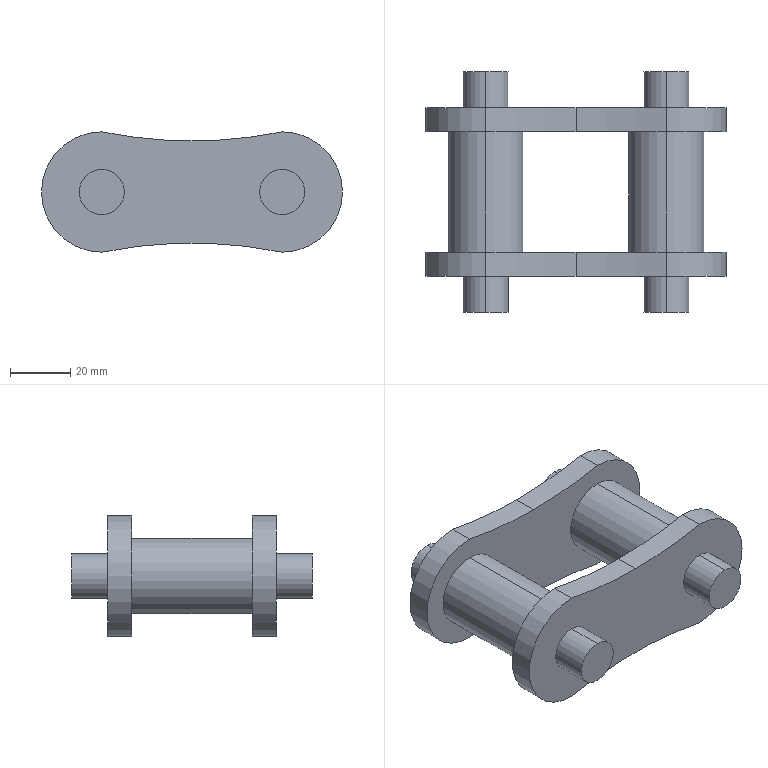Part | SolidWorks | features ICE 2, LPattern 2, RefPoint 2, Extrusion 1 | 1 solid | 30 faces | box 100 x 80 x 40 mm | volume 102371 mm3 | cylinder 22 | plane 8 | commonest cylinder face diameters 15 x8 300 x6 25 x4 40 x4
STEP:
#1=CARTESIAN_POINT('',(0.,0.,-7.5));
#2=VERTEX_POINT('',#1);
#3=CARTESIAN_POINT('',(0.,0.,7.5));
#4=VERTEX_POINT('',#3);
#5=CARTESIAN_POINT('',(0.,0.,0.));
#6=DIRECTION('',(0.,-1.,0.));
#7=DIRECTION('',(0.,0.,1.));
#8=AXIS2_PLACEMENT_3D('',#5,#6,#7);
#9=CIRCLE('',#8,7.5);
#10=EDGE_CURVE('',#2,#4,#9,.T.);
#11=ORIENTED_EDGE('',*,*,#10,.T.);
#12=CARTESIAN_POINT('',(0.,-12.,7.5));
#13=VERTEX_POINT('',#12);
#14=CARTESIAN_POINT('',(0.,0.,7.5));
#15=DIRECTION('',(0.,-1.,0.));
#16=VECTOR('',#15,1000.);
#17=LINE('',#14,#16);
#18=EDGE_CURVE('',#4,#13,#17,.T.);
#19=ORIENTED_EDGE('',*,*,#18,.T.);
#20=CARTESIAN_POINT('',(0.,-12.,-7.5));
#21=VERTEX_POINT('',#20);
#22=CARTESIAN_POINT('',(0.,-12.,0.));
#23=DIRECTION('',(0.,1.,0.));
#24=DIRECTION('',(0.,0.,1.));
#25=AXIS2_PLACEMENT_3D('',#22,#23,#24);
#26=CIRCLE('',#25,7.5);
#27=EDGE_CURVE('',#13,#21,#26,.T.);
#28=ORIENTED_EDGE('',*,*,#27,.T.);
#29=CARTESIAN_POINT('',(0.,0.,-7.5));
#30=DIRECTION('',(0.,-1.,0.));
#31=VECTOR('',#30,1000.);
#32=LINE('',#29,#31);
#33=EDGE_CURVE('',#2,#21,#32,.T.);
#34=ORIENTED_EDGE('',*,*,#33,.F.);
#35=EDGE_LOOP('',(#11,#19,#28,#34));
#36=FACE_OUTER_BOUND('',#35,.T.);
#37=CARTESIAN_POINT('',(0.,0.,0.));
#38=DIRECTION('',(0.,-1.,0.));
#39=DIRECTION('',(0.,0.,-1.));
#40=AXIS2_PLACEMENT_3D('',#37,#38,#39);
#41=CYLINDRICAL_SURFACE('',#40,7.5);
#42=ADVANCED_FACE('',(#36),#41,.T.);
#43=CARTESIAN_POINT('',(60.,0.,-7.5));
#44=VERTEX_POINT('',#43);
#45=CARTESIAN_POINT('',(60.,0.,7.5));
#46=VERTEX_POINT('',#45);
#47=CARTESIAN_POINT('',(60.,0.,0.));
#48=DIRECTION('',(0.,-1.,0.));
#49=DIRECTION('',(0.,0.,1.));
#50=AXIS2_PLACEMENT_3D('',#47,#48,#49);
#51=CIRCLE('',#50,7.5);
#52=EDGE_CURVE('',#44,#46,#51,.T.);
#53=ORIENTED_EDGE('',*,*,#52,.T.);
#54=CARTESIAN_POINT('',(60.,-12.,7.5));
#55=VERTEX_POINT('',#54);
#56=CARTESIAN_POINT('',(60.,0.,7.5));
#57=DIRECTION('',(0.,-1.,0.));
#58=VECTOR('',#57,1000.);
#59=LINE('',#56,#58);
#60=EDGE_CURVE('',#46,#55,#59,.T.);
#61=ORIENTED_EDGE('',*,*,#60,.T.);
#62=CARTESIAN_POINT('',(60.,-12.,-7.5));
#63=VERTEX_POINT('',#62);
#64=CARTESIAN_POINT('',(60.,-12.,0.));
#65=DIRECTION('',(0.,1.,0.));
#66=DIRECTION('',(0.,0.,1.));
#67=AXIS2_PLACEMENT_3D('',#64,#65,#66);
#68=CIRCLE('',#67,7.5);
#69=EDGE_CURVE('',#55,#63,#68,.T.);
#70=ORIENTED_EDGE('',*,*,#69,.T.);
#71=CARTESIAN_POINT('',(60.,0.,-7.5));
#72=DIRECTION('',(0.,-1.,0.));
#73=VECTOR('',#72,1000.);
#74=LINE('',#71,#73);
#75=EDGE_CURVE('',#44,#63,#74,.T.);
#76=ORIENTED_EDGE('',*,*,#75,.F.);
#77=EDGE_LOOP('',(#53,#61,#70,#76));
#78=FACE_OUTER_BOUND('',#77,.T.);
#79=CARTESIAN_POINT('',(60.,0.,0.));
#80=DIRECTION('',(0.,-1.,0.));
#81=DIRECTION('',(0.,0.,-1.));
#82=AXIS2_PLACEMENT_3D('',#79,#80,#81);
#83=CYLINDRICAL_SURFACE('',#82,7.5);
#84=ADVANCED_FACE('',(#78),#83,.T.);
#85=CARTESIAN_POINT('',(0.,68.,7.5));
#86=VERTEX_POINT('',#85);
#87=CARTESIAN_POINT('',(0.,68.,-7.5));
#88=VERTEX_POINT('',#87);
#89=CARTESIAN_POINT('',(0.,68.,0.));
#90=DIRECTION('',(0.,1.,0.));
#91=DIRECTION('',(0.,0.,1.));
#92=AXIS2_PLACEMENT_3D('',#89,#90,#91);
#93=CIRCLE('',#92,7.5);
#94=EDGE_CURVE('',#86,#88,#93,.T.);
#95=ORIENTED_EDGE('',*,*,#94,.F.);
#96=CARTESIAN_POINT('',(0.,56.,7.5));
#97=VERTEX_POINT('',#96);
#98=CARTESIAN_POINT('',(0.,68.,7.5));
#99=DIRECTION('',(0.,-1.,0.));
#100=VECTOR('',#99,1000.);
#101=LINE('',#98,#100);
#102=EDGE_CURVE('',#86,#97,#101,.T.);
#103=ORIENTED_EDGE('',*,*,#102,.T.);
#104=CARTESIAN_POINT('',(0.,56.,-7.5));
#105=VERTEX_POINT('',#104);
#106=CARTESIAN_POINT('',(0.,56.,0.));
#107=DIRECTION('',(0.,1.,0.));
#108=DIRECTION('',(0.,0.,1.));
#109=AXIS2_PLACEMENT_3D('',#106,#107,#108);
#110=CIRCLE('',#109,7.5);
#111=EDGE_CURVE('',#97,#105,#110,.T.);
#112=ORIENTED_EDGE('',*,*,#111,.T.);
#113=CARTESIAN_POINT('',(0.,68.,-7.5));
#114=DIRECTION('',(0.,-1.,0.));
#115=VECTOR('',#114,1000.);
#116=LINE('',#113,#115);
#117=EDGE_CURVE('',#88,#105,#116,.T.);
#118=ORIENTED_EDGE('',*,*,#117,.F.);
#119=EDGE_LOOP('',(#95,#103,#112,#118));
#120=FACE_OUTER_BOUND('',#119,.T.);
#121=CARTESIAN_POINT('',(0.,68.,0.));
#122=DIRECTION('',(0.,-1.,0.));
#123=DIRECTION('',(0.,0.,-1.));
#124=AXIS2_PLACEMENT_3D('',#121,#122,#123);
#125=CYLINDRICAL_SURFACE('',#124,7.5);
#126=ADVANCED_FACE('',(#120),#125,.T.);
#127=CARTESIAN_POINT('',(60.,68.,7.5));
#128=VERTEX_POINT('',#127);
#129=CARTESIAN_POINT('',(60.,68.,-7.5));
#130=VERTEX_POINT('',#129);
#131=CARTESIAN_POINT('',(60.,68.,0.));
#132=DIRECTION('',(0.,1.,0.));
#133=DIRECTION('',(0.,0.,1.));
#134=AXIS2_PLACEMENT_3D('',#131,#132,#133);
#135=CIRCLE('',#134,7.5);
#136=EDGE_CURVE('',#128,#130,#135,.T.);
#137=ORIENTED_EDGE('',*,*,#136,.F.);
#138=CARTESIAN_POINT('',(60.,56.,7.5));
#139=VERTEX_POINT('',#138);
#140=CARTESIAN_POINT('',(60.,68.,7.5));
#141=DIRECTION('',(0.,-1.,0.));
#142=VECTOR('',#141,1000.);
#143=LINE('',#140,#142);
#144=EDGE_CURVE('',#128,#139,#143,.T.);
#145=ORIENTED_EDGE('',*,*,#144,.T.);
#146=CARTESIAN_POINT('',(60.,56.,-7.5));
#147=VERTEX_POINT('',#146);
#148=CARTESIAN_POINT('',(60.,56.,0.));
#149=DIRECTION('',(0.,1.,0.));
#150=DIRECTION('',(0.,0.,1.));
#151=AXIS2_PLACEMENT_3D('',#148,#149,#150);
#152=CIRCLE('',#151,7.5);
#153=EDGE_CURVE('',#139,#147,#152,.T.);
#154=ORIENTED_EDGE('',*,*,#153,.T.);
#155=CARTESIAN_POINT('',(60.,68.,-7.5));
#156=DIRECTION('',(0.,-1.,0.));
#157=VECTOR('',#156,1000.);
#158=LINE('',#155,#157);
#159=EDGE_CURVE('',#130,#147,#158,.T.);
#160=ORIENTED_EDGE('',*,*,#159,.F.);
#161=EDGE_LOOP('',(#137,#145,#154,#160));
#162=FACE_OUTER_BOUND('',#161,.T.);
#163=CARTESIAN_POINT('',(60.,68.,0.));
#164=DIRECTION('',(0.,-1.,0.));
#165=DIRECTION('',(0.,0.,-1.));
#166=AXIS2_PLACEMENT_3D('',#163,#164,#165);
#167=CYLINDRICAL_SURFACE('',#166,7.5);
#168=ADVANCED_FACE('',(#162),#167,.T.);
#169=CARTESIAN_POINT('',(30.,56.,16.969));
#170=VERTEX_POINT('',#169);
#171=CARTESIAN_POINT('',(60.,56.,20.));
#172=VERTEX_POINT('',#171);
#173=CARTESIAN_POINT('',(30.,56.,166.969));
#174=DIRECTION('',(0.,-1.,0.));
#175=DIRECTION('',(0.,0.,-1.));
#176=AXIS2_PLACEMENT_3D('',#173,#174,#175);
#177=CIRCLE('',#176,150.);
#178=EDGE_CURVE('',#170,#172,#177,.T.);
#179=ORIENTED_EDGE('',*,*,#178,.F.);
#180=CARTESIAN_POINT('',(30.,48.,16.969));
#181=VERTEX_POINT('',#180);
#182=CARTESIAN_POINT('',(30.,56.,16.969));
#183=DIRECTION('',(0.,-1.,0.));
#184=VECTOR('',#183,1000.);
#185=LINE('',#182,#184);
#186=EDGE_CURVE('',#170,#181,#185,.T.);
#187=ORIENTED_EDGE('',*,*,#186,.T.);
#188=CARTESIAN_POINT('',(60.,48.,20.));
#189=VERTEX_POINT('',#188);
#190=CARTESIAN_POINT('',(30.,48.,166.969));
#191=DIRECTION('',(0.,-1.,0.));
#192=DIRECTION('',(0.,0.,-1.));
#193=AXIS2_PLACEMENT_3D('',#190,#191,#192);
#194=CIRCLE('',#193,150.);
#195=EDGE_CURVE('',#181,#189,#194,.T.);
#196=ORIENTED_EDGE('',*,*,#195,.T.);
#197=CARTESIAN_POINT('',(60.,56.,20.));
#198=DIRECTION('',(0.,-1.,0.));
#199=VECTOR('',#198,1000.);
#200=LINE('',#197,#199);
#201=EDGE_CURVE('',#172,#189,#200,.T.);
#202=ORIENTED_EDGE('',*,*,#201,.F.);
#203=EDGE_LOOP('',(#179,#187,#196,#202));
#204=FACE_OUTER_BOUND('',#203,.T.);
#205=CARTESIAN_POINT('',(30.,56.,166.969));
#206=DIRECTION('',(0.,-1.,0.));
#207=DIRECTION('',(0.,0.,-1.));
#208=AXIS2_PLACEMENT_3D('',#205,#206,#207);
#209=CYLINDRICAL_SURFACE('',#208,150.);
#210=ADVANCED_FACE('',(#204),#209,.F.);
#211=CARTESIAN_POINT('',(0.,48.,12.5));
#212=VERTEX_POINT('',#211);
#213=CARTESIAN_POINT('',(0.,48.,-12.5));
#214=VERTEX_POINT('',#213);
#215=CARTESIAN_POINT('',(0.,48.,0.));
#216=DIRECTION('',(0.,1.,0.));
#217=DIRECTION('',(0.,0.,1.));
#218=AXIS2_PLACEMENT_3D('',#215,#216,#217);
#219=CIRCLE('',#218,12.5);
#220=EDGE_CURVE('',#212,#214,#219,.T.);
#221=ORIENTED_EDGE('',*,*,#220,.F.);
#222=CARTESIAN_POINT('',(0.,8.,12.5));
#223=VERTEX_POINT('',#222);
#224=CARTESIAN_POINT('',(0.,48.,12.5));
#225=DIRECTION('',(0.,-1.,0.));
#226=VECTOR('',#225,1000.);
#227=LINE('',#224,#226);
#228=EDGE_CURVE('',#212,#223,#227,.T.);
#229=ORIENTED_EDGE('',*,*,#228,.T.);
#230=CARTESIAN_POINT('',(0.,8.,-12.5));
#231=VERTEX_POINT('',#230);
#232=CARTESIAN_POINT('',(0.,8.,0.));
#233=DIRECTION('',(0.,1.,0.));
#234=DIRECTION('',(0.,0.,1.));
#235=AXIS2_PLACEMENT_3D('',#232,#233,#234);
#236=CIRCLE('',#235,12.5);
#237=EDGE_CURVE('',#223,#231,#236,.T.);
#238=ORIENTED_EDGE('',*,*,#237,.T.);
#239=CARTESIAN_POINT('',(0.,48.,-12.5));
#240=DIRECTION('',(0.,-1.,0.));
#241=VECTOR('',#240,1000.);
#242=LINE('',#239,#241);
#243=EDGE_CURVE('',#214,#231,#242,.T.);
#244=ORIENTED_EDGE('',*,*,#243,.F.);
#245=EDGE_LOOP('',(#221,#229,#238,#244));
#246=FACE_OUTER_BOUND('',#245,.T.);
#247=CARTESIAN_POINT('',(0.,48.,0.));
#248=DIRECTION('',(0.,-1.,0.));
#249=DIRECTION('',(0.,0.,-1.));
#250=AXIS2_PLACEMENT_3D('',#247,#248,#249);
#251=CYLINDRICAL_SURFACE('',#250,12.5);
#252=ADVANCED_FACE('',(#246),#251,.T.);
#253=CARTESIAN_POINT('',(60.,48.,12.5));
#254=VERTEX_POINT('',#253);
#255=CARTESIAN_POINT('',(60.,48.,-12.5));
#256=VERTEX_POINT('',#255);
#257=CARTESIAN_POINT('',(60.,48.,0.));
#258=DIRECTION('',(0.,1.,0.));
#259=DIRECTION('',(0.,0.,1.));
#260=AXIS2_PLACEMENT_3D('',#257,#258,#259);
#261=CIRCLE('',#260,12.5);
#262=EDGE_CURVE('',#254,#256,#261,.T.);
#263=ORIENTED_EDGE('',*,*,#262,.F.);
#264=CARTESIAN_POINT('',(60.,8.,12.5));
#265=VERTEX_POINT('',#264);
#266=CARTESIAN_POINT('',(60.,48.,12.5));
#267=DIRECTION('',(0.,-1.,0.));
#268=VECTOR('',#267,1000.);
#269=LINE('',#266,#268);
#270=EDGE_CURVE('',#254,#265,#269,.T.);
#271=ORIENTED_EDGE('',*,*,#270,.T.);
#272=CARTESIAN_POINT('',(60.,8.,-12.5));
#273=VERTEX_POINT('',#272);
#274=CARTESIAN_POINT('',(60.,8.,0.));
#275=DIRECTION('',(0.,1.,0.));
#276=DIRECTION('',(0.,0.,1.));
#277=AXIS2_PLACEMENT_3D('',#274,#275,#276);
#278=CIRCLE('',#277,12.5);
#279=EDGE_CURVE('',#265,#273,#278,.T.);
#280=ORIENTED_EDGE('',*,*,#279,.T.);
#281=CARTESIAN_POINT('',(60.,48.,-12.5));
#282=DIRECTION('',(0.,-1.,0.));
#283=VECTOR('',#282,1000.);
#284=LINE('',#281,#283);
#285=EDGE_CURVE('',#256,#273,#284,.T.);
#286=ORIENTED_EDGE('',*,*,#285,.F.);
#287=EDGE_LOOP('',(#263,#271,#280,#286));
#288=FACE_OUTER_BOUND('',#287,.T.);
#289=CARTESIAN_POINT('',(60.,48.,0.));
#290=DIRECTION('',(0.,-1.,0.));
#291=DIRECTION('',(0.,0.,-1.));
#292=AXIS2_PLACEMENT_3D('',#289,#290,#291);
#293=CYLINDRICAL_SURFACE('',#292,12.5);
#294=ADVANCED_FACE('',(#288),#293,.T.);
#295=CARTESIAN_POINT('',(30.,8.,16.969));
#296=VERTEX_POINT('',#295);
#297=CARTESIAN_POINT('',(60.,8.,20.));
#298=VERTEX_POINT('',#297);
#299=CARTESIAN_POINT('',(30.,8.,166.969));
#300=DIRECTION('',(0.,-1.,0.));
#301=DIRECTION('',(0.,0.,-1.));
#302=AXIS2_PLACEMENT_3D('',#299,#300,#301);
#303=CIRCLE('',#302,150.);
#304=EDGE_CURVE('',#296,#298,#303,.T.);
#305=ORIENTED_EDGE('',*,*,#304,.F.);
#306=CARTESIAN_POINT('',(30.,0.,16.969));
#307=VERTEX_POINT('',#306);
#308=CARTESIAN_POINT('',(30.,8.,16.969));
#309=DIRECTION('',(0.,-1.,0.));
#310=VECTOR('',#309,1000.);
#311=LINE('',#308,#310);
#312=EDGE_CURVE('',#296,#307,#311,.T.);
#313=ORIENTED_EDGE('',*,*,#312,.T.);
#314=CARTESIAN_POINT('',(60.,0.,20.));
#315=VERTEX_POINT('',#314);
#316=CARTESIAN_POINT('',(30.,0.,166.969));
#317=DIRECTION('',(0.,-1.,0.));
#318=DIRECTION('',(0.,0.,-1.));
#319=AXIS2_PLACEMENT_3D('',#316,#317,#318);
#320=CIRCLE('',#319,150.);
#321=EDGE_CURVE('',#307,#315,#320,.T.);
#322=ORIENTED_EDGE('',*,*,#321,.T.);
#323=CARTESIAN_POINT('',(60.,8.,20.));
#324=DIRECTION('',(0.,-1.,0.));
#325=VECTOR('',#324,1000.);
#326=LINE('',#323,#325);
#327=EDGE_CURVE('',#298,#315,#326,.T.);
#328=ORIENTED_EDGE('',*,*,#327,.F.);
#329=EDGE_LOOP('',(#305,#313,#322,#328));
#330=FACE_OUTER_BOUND('',#329,.T.);
#331=CARTESIAN_POINT('',(30.,8.,166.969));
#332=DIRECTION('',(0.,-1.,0.));
#333=DIRECTION('',(0.,0.,-1.));
#334=AXIS2_PLACEMENT_3D('',#331,#332,#333);
#335=CYLINDRICAL_SURFACE('',#334,150.);
#336=ADVANCED_FACE('',(#330),#335,.F.);
#337=CARTESIAN_POINT('',(60.,0.,-20.));
#338=VERTEX_POINT('',#337);
#339=CARTESIAN_POINT('',(0.,0.,-20.));
#340=VERTEX_POINT('',#339);
#341=CARTESIAN_POINT('',(30.,0.,-166.969));
#342=DIRECTION('',(0.,-1.,0.));
#343=DIRECTION('',(0.,0.,1.));
#344=AXIS2_PLACEMENT_3D('',#341,#342,#343);
#345=CIRCLE('',#344,150.);
#346=EDGE_CURVE('',#338,#340,#345,.T.);
#347=ORIENTED_EDGE('',*,*,#346,.T.);
#348=CARTESIAN_POINT('',(0.,8.,-20.));
#349=VERTEX_POINT('',#348);
#350=CARTESIAN_POINT('',(0.,8.,-20.));
#351=DIRECTION('',(0.,-1.,0.));
#352=VECTOR('',#351,1000.);
#353=LINE('',#350,#352);
#354=EDGE_CURVE('',#349,#340,#353,.T.);
#355=ORIENTED_EDGE('',*,*,#354,.F.);
#356=CARTESIAN_POINT('',(60.,8.,-20.));
#357=VERTEX_POINT('',#356);
#358=CARTESIAN_POINT('',(30.,8.,-166.969));
#359=DIRECTION('',(0.,-1.,0.));
#360=DIRECTION('',(0.,0.,1.));
#361=AXIS2_PLACEMENT_3D('',#358,#359,#360);
#362=CIRCLE('',#361,150.);
#363=EDGE_CURVE('',#357,#349,#362,.T.);
#364=ORIENTED_EDGE('',*,*,#363,.F.);
#365=CARTESIAN_POINT('',(60.,8.,-20.));
#366=DIRECTION('',(0.,-1.,0.));
#367=VECTOR('',#366,1000.);
#368=LINE('',#365,#367);
#369=EDGE_CURVE('',#357,#338,#368,.T.);
#370=ORIENTED_EDGE('',*,*,#369,.T.);
#371=EDGE_LOOP('',(#347,#355,#364,#370));
#372=FACE_OUTER_BOUND('',#371,.T.);
#373=CARTESIAN_POINT('',(30.,8.,-166.969));
#374=DIRECTION('',(0.,-1.,0.));
#375=DIRECTION('',(0.,0.,-1.));
#376=AXIS2_PLACEMENT_3D('',#373,#374,#375);
#377=CYLINDRICAL_SURFACE('',#376,150.);
#378=ADVANCED_FACE('',(#372),#377,.F.);
#379=CARTESIAN_POINT('',(0.,0.,20.));
#380=VERTEX_POINT('',#379);
#381=CARTESIAN_POINT('',(0.,0.,0.));
#382=DIRECTION('',(0.,1.,0.));
#383=DIRECTION('',(0.,0.,1.));
#384=AXIS2_PLACEMENT_3D('',#381,#382,#383);
#385=CIRCLE('',#384,20.);
#386=EDGE_CURVE('',#340,#380,#385,.T.);
#387=ORIENTED_EDGE('',*,*,#386,.T.);
#388=CARTESIAN_POINT('',(0.,8.,20.));
#389=VERTEX_POINT('',#388);
#390=CARTESIAN_POINT('',(0.,8.,20.));
#391=DIRECTION('',(0.,-1.,0.));
#392=VECTOR('',#391,1000.);
#393=LINE('',#390,#392);
#394=EDGE_CURVE('',#389,#380,#393,.T.);
#395=ORIENTED_EDGE('',*,*,#394,.F.);
#396=CARTESIAN_POINT('',(0.,8.,0.));
#397=DIRECTION('',(0.,1.,0.));
#398=DIRECTION('',(0.,0.,1.));
#399=AXIS2_PLACEMENT_3D('',#396,#397,#398);
#400=CIRCLE('',#399,20.);
#401=EDGE_CURVE('',#349,#389,#400,.T.);
#402=ORIENTED_EDGE('',*,*,#401,.F.);
#403=ORIENTED_EDGE('',*,*,#354,.T.);
#404=EDGE_LOOP('',(#387,#395,#402,#403));
#405=FACE_OUTER_BOUND('',#404,.T.);
#406=CARTESIAN_POINT('',(0.,8.,0.));
#407=DIRECTION('',(0.,-1.,0.));
#408=DIRECTION('',(0.,0.,-1.));
#409=AXIS2_PLACEMENT_3D('',#406,#407,#408);
#410=CYLINDRICAL_SURFACE('',#409,20.);
#411=ADVANCED_FACE('',(#405),#410,.T.);
#412=ORIENTED_EDGE('',*,*,#312,.F.);
#413=CARTESIAN_POINT('',(30.,8.,166.969));
#414=DIRECTION('',(0.,-1.,0.));
#415=DIRECTION('',(0.,0.,-1.));
#416=AXIS2_PLACEMENT_3D('',#413,#414,#415);
#417=CIRCLE('',#416,150.);
#418=EDGE_CURVE('',#389,#296,#417,.T.);
#419=ORIENTED_EDGE('',*,*,#418,.F.);
#420=ORIENTED_EDGE('',*,*,#394,.T.);
#421=CARTESIAN_POINT('',(30.,0.,166.969));
#422=DIRECTION('',(0.,-1.,0.));
#423=DIRECTION('',(0.,0.,-1.));
#424=AXIS2_PLACEMENT_3D('',#421,#422,#423);
#425=CIRCLE('',#424,150.);
#426=EDGE_CURVE('',#380,#307,#425,.T.);
#427=ORIENTED_EDGE('',*,*,#426,.T.);
#428=EDGE_LOOP('',(#412,#419,#420,#427));
#429=FACE_OUTER_BOUND('',#428,.T.);
#430=CARTESIAN_POINT('',(30.,8.,166.969));
#431=DIRECTION('',(0.,-1.,0.));
#432=DIRECTION('',(0.,0.,-1.));
#433=AXIS2_PLACEMENT_3D('',#430,#431,#432);
#434=CYLINDRICAL_SURFACE('',#433,150.);
#435=ADVANCED_FACE('',(#429),#434,.F.);
#436=CARTESIAN_POINT('',(60.,0.,0.));
#437=DIRECTION('',(0.,1.,0.));
#438=DIRECTION('',(0.,0.,1.));
#439=AXIS2_PLACEMENT_3D('',#436,#437,#438);
#440=CIRCLE('',#439,20.);
#441=EDGE_CURVE('',#315,#338,#440,.T.);
#442=ORIENTED_EDGE('',*,*,#441,.T.);
#443=ORIENTED_EDGE('',*,*,#369,.F.);
#444=CARTESIAN_POINT('',(60.,8.,0.));
#445=DIRECTION('',(0.,1.,0.));
#446=DIRECTION('',(0.,0.,1.));
#447=AXIS2_PLACEMENT_3D('',#444,#445,#446);
#448=CIRCLE('',#447,20.);
#449=EDGE_CURVE('',#298,#357,#448,.T.);
#450=ORIENTED_EDGE('',*,*,#449,.F.);
#451=ORIENTED_EDGE('',*,*,#327,.T.);
#452=EDGE_LOOP('',(#442,#443,#450,#451));
#453=FACE_OUTER_BOUND('',#452,.T.);
#454=CARTESIAN_POINT('',(60.,8.,0.));
#455=DIRECTION('',(0.,-1.,0.));
#456=DIRECTION('',(0.,0.,-1.));
#457=AXIS2_PLACEMENT_3D('',#454,#455,#456);
#458=CYLINDRICAL_SURFACE('',#457,20.);
#459=ADVANCED_FACE('',(#453),#458,.T.);
#460=CARTESIAN_POINT('',(0.,8.,0.));
#461=DIRECTION('',(0.,1.,0.));
#462=DIRECTION('',(0.,0.,1.));
#463=AXIS2_PLACEMENT_3D('',#460,#461,#462);
#464=CIRCLE('',#463,12.5);
#465=EDGE_CURVE('',#231,#223,#464,.T.);
#466=ORIENTED_EDGE('',*,*,#465,.F.);
#467=ORIENTED_EDGE('',*,*,#237,.F.);
#468=EDGE_LOOP('',(#466,#467));
#469=FACE_BOUND('',#468,.T.);
#470=CARTESIAN_POINT('',(60.,8.,0.));
#471=DIRECTION('',(0.,1.,0.));
#472=DIRECTION('',(0.,0.,1.));
#473=AXIS2_PLACEMENT_3D('',#470,#471,#472);
#474=CIRCLE('',#473,12.5);
#475=EDGE_CURVE('',#273,#265,#474,.T.);
#476=ORIENTED_EDGE('',*,*,#475,.F.);
#477=ORIENTED_EDGE('',*,*,#279,.F.);
#478=EDGE_LOOP('',(#476,#477));
#479=FACE_BOUND('',#478,.T.);
#480=ORIENTED_EDGE('',*,*,#363,.T.);
#481=ORIENTED_EDGE('',*,*,#401,.T.);
#482=ORIENTED_EDGE('',*,*,#418,.T.);
#483=ORIENTED_EDGE('',*,*,#304,.T.);
#484=ORIENTED_EDGE('',*,*,#449,.T.);
#485=EDGE_LOOP('',(#480,#481,#482,#483,#484));
#486=FACE_OUTER_BOUND('',#485,.T.);
#487=CARTESIAN_POINT('',(45.,8.,-83.485));
#488=DIRECTION('',(0.,1.,0.));
#489=DIRECTION('',(0.,0.,1.));
#490=AXIS2_PLACEMENT_3D('',#487,#488,#489);
#491=PLANE('',#490);
#492=ADVANCED_FACE('',(#469,#479,#486),#491,.T.);
#493=ORIENTED_EDGE('',*,*,#10,.F.);
#494=CARTESIAN_POINT('',(0.,0.,0.));
#495=DIRECTION('',(0.,-1.,0.));
#496=DIRECTION('',(0.,0.,1.));
#497=AXIS2_PLACEMENT_3D('',#494,#495,#496);
#498=CIRCLE('',#497,7.5);
#499=EDGE_CURVE('',#4,#2,#498,.T.);
#500=ORIENTED_EDGE('',*,*,#499,.F.);
#501=EDGE_LOOP('',(#493,#500));
#502=FACE_BOUND('',#501,.T.);
#503=ORIENTED_EDGE('',*,*,#52,.F.);
#504=CARTESIAN_POINT('',(60.,0.,0.));
#505=DIRECTION('',(0.,-1.,0.));
#506=DIRECTION('',(0.,0.,1.));
#507=AXIS2_PLACEMENT_3D('',#504,#505,#506);
#508=CIRCLE('',#507,7.5);
#509=EDGE_CURVE('',#46,#44,#508,.T.);
#510=ORIENTED_EDGE('',*,*,#509,.F.);
#511=EDGE_LOOP('',(#503,#510));
#512=FACE_BOUND('',#511,.T.);
#513=ORIENTED_EDGE('',*,*,#346,.F.);
#514=ORIENTED_EDGE('',*,*,#441,.F.);
#515=ORIENTED_EDGE('',*,*,#321,.F.);
#516=ORIENTED_EDGE('',*,*,#426,.F.);
#517=ORIENTED_EDGE('',*,*,#386,.F.);
#518=EDGE_LOOP('',(#513,#514,#515,#516,#517));
#519=FACE_OUTER_BOUND('',#518,.T.);
#520=CARTESIAN_POINT('',(45.,0.,-83.485));
#521=DIRECTION('',(0.,1.,0.));
#522=DIRECTION('',(0.,0.,1.));
#523=AXIS2_PLACEMENT_3D('',#520,#521,#522);
#524=PLANE('',#523);
#525=ADVANCED_FACE('',(#502,#512,#519),#524,.F.);
#526=ORIENTED_EDGE('',*,*,#270,.F.);
#527=CARTESIAN_POINT('',(60.,48.,0.));
#528=DIRECTION('',(0.,1.,0.));
#529=DIRECTION('',(0.,0.,1.));
#530=AXIS2_PLACEMENT_3D('',#527,#528,#529);
#531=CIRCLE('',#530,12.5);
#532=EDGE_CURVE('',#256,#254,#531,.T.);
#533=ORIENTED_EDGE('',*,*,#532,.F.);
#534=ORIENTED_EDGE('',*,*,#285,.T.);
#535=ORIENTED_EDGE('',*,*,#475,.T.);
#536=EDGE_LOOP('',(#526,#533,#534,#535));
#537=FACE_OUTER_BOUND('',#536,.T.);
#538=CARTESIAN_POINT('',(60.,48.,0.));
#539=DIRECTION('',(0.,-1.,0.));
#540=DIRECTION('',(0.,0.,-1.));
#541=AXIS2_PLACEMENT_3D('',#538,#539,#540);
#542=CYLINDRICAL_SURFACE('',#541,12.5);
#543=ADVANCED_FACE('',(#537),#542,.T.);
#544=ORIENTED_EDGE('',*,*,#228,.F.);
#545=CARTESIAN_POINT('',(0.,48.,0.));
#546=DIRECTION('',(0.,1.,0.));
#547=DIRECTION('',(0.,0.,1.));
#548=AXIS2_PLACEMENT_3D('',#545,#546,#547);
#549=CIRCLE('',#548,12.5);
#550=EDGE_CURVE('',#214,#212,#549,.T.);
#551=ORIENTED_EDGE('',*,*,#550,.F.);
#552=ORIENTED_EDGE('',*,*,#243,.T.);
#553=ORIENTED_EDGE('',*,*,#465,.T.);
#554=EDGE_LOOP('',(#544,#551,#552,#553));
#555=FACE_OUTER_BOUND('',#554,.T.);
#556=CARTESIAN_POINT('',(0.,48.,0.));
#557=DIRECTION('',(0.,-1.,0.));
#558=DIRECTION('',(0.,0.,-1.));
#559=AXIS2_PLACEMENT_3D('',#556,#557,#558);
#560=CYLINDRICAL_SURFACE('',#559,12.5);
#561=ADVANCED_FACE('',(#555),#560,.T.);
#562=CARTESIAN_POINT('',(60.,48.,-20.));
#563=VERTEX_POINT('',#562);
#564=CARTESIAN_POINT('',(0.,48.,-20.));
#565=VERTEX_POINT('',#564);
#566=CARTESIAN_POINT('',(30.,48.,-166.969));
#567=DIRECTION('',(0.,-1.,0.));
#568=DIRECTION('',(0.,0.,1.));
#569=AXIS2_PLACEMENT_3D('',#566,#567,#568);
#570=CIRCLE('',#569,150.);
#571=EDGE_CURVE('',#563,#565,#570,.T.);
#572=ORIENTED_EDGE('',*,*,#571,.T.);
#573=CARTESIAN_POINT('',(0.,56.,-20.));
#574=VERTEX_POINT('',#573);
#575=CARTESIAN_POINT('',(0.,56.,-20.));
#576=DIRECTION('',(0.,-1.,0.));
#577=VECTOR('',#576,1000.);
#578=LINE('',#575,#577);
#579=EDGE_CURVE('',#574,#565,#578,.T.);
#580=ORIENTED_EDGE('',*,*,#579,.F.);
#581=CARTESIAN_POINT('',(60.,56.,-20.));
#582=VERTEX_POINT('',#581);
#583=CARTESIAN_POINT('',(30.,56.,-166.969));
#584=DIRECTION('',(0.,-1.,0.));
#585=DIRECTION('',(0.,0.,1.));
#586=AXIS2_PLACEMENT_3D('',#583,#584,#585);
#587=CIRCLE('',#586,150.);
#588=EDGE_CURVE('',#582,#574,#587,.T.);
#589=ORIENTED_EDGE('',*,*,#588,.F.);
#590=CARTESIAN_POINT('',(60.,56.,-20.));
#591=DIRECTION('',(0.,-1.,0.));
#592=VECTOR('',#591,1000.);
#593=LINE('',#590,#592);
#594=EDGE_CURVE('',#582,#563,#593,.T.);
#595=ORIENTED_EDGE('',*,*,#594,.T.);
#596=EDGE_LOOP('',(#572,#580,#589,#595));
#597=FACE_OUTER_BOUND('',#596,.T.);
#598=CARTESIAN_POINT('',(30.,56.,-166.969));
#599=DIRECTION('',(0.,-1.,0.));
#600=DIRECTION('',(0.,0.,-1.));
#601=AXIS2_PLACEMENT_3D('',#598,#599,#600);
#602=CYLINDRICAL_SURFACE('',#601,150.);
#603=ADVANCED_FACE('',(#597),#602,.F.);
#604=CARTESIAN_POINT('',(0.,48.,20.));
#605=VERTEX_POINT('',#604);
#606=CARTESIAN_POINT('',(0.,48.,0.));
#607=DIRECTION('',(0.,1.,0.));
#608=DIRECTION('',(0.,0.,1.));
#609=AXIS2_PLACEMENT_3D('',#606,#607,#608);
#610=CIRCLE('',#609,20.);
#611=EDGE_CURVE('',#565,#605,#610,.T.);
#612=ORIENTED_EDGE('',*,*,#611,.T.);
#613=CARTESIAN_POINT('',(0.,56.,20.));
#614=VERTEX_POINT('',#613);
#615=CARTESIAN_POINT('',(0.,56.,20.));
#616=DIRECTION('',(0.,-1.,0.));
#617=VECTOR('',#616,1000.);
#618=LINE('',#615,#617);
#619=EDGE_CURVE('',#614,#605,#618,.T.);
#620=ORIENTED_EDGE('',*,*,#619,.F.);
#621=CARTESIAN_POINT('',(0.,56.,0.));
#622=DIRECTION('',(0.,1.,0.));
#623=DIRECTION('',(0.,0.,1.));
#624=AXIS2_PLACEMENT_3D('',#621,#622,#623);
#625=CIRCLE('',#624,20.);
#626=EDGE_CURVE('',#574,#614,#625,.T.);
#627=ORIENTED_EDGE('',*,*,#626,.F.);
#628=ORIENTED_EDGE('',*,*,#579,.T.);
#629=EDGE_LOOP('',(#612,#620,#627,#628));
#630=FACE_OUTER_BOUND('',#629,.T.);
#631=CARTESIAN_POINT('',(0.,56.,0.));
#632=DIRECTION('',(0.,-1.,0.));
#633=DIRECTION('',(0.,0.,-1.));
#634=AXIS2_PLACEMENT_3D('',#631,#632,#633);
#635=CYLINDRICAL_SURFACE('',#634,20.);
#636=ADVANCED_FACE('',(#630),#635,.T.);
#637=ORIENTED_EDGE('',*,*,#186,.F.);
#638=CARTESIAN_POINT('',(30.,56.,166.969));
#639=DIRECTION('',(0.,-1.,0.));
#640=DIRECTION('',(0.,0.,-1.));
#641=AXIS2_PLACEMENT_3D('',#638,#639,#640);
#642=CIRCLE('',#641,150.);
#643=EDGE_CURVE('',#614,#170,#642,.T.);
#644=ORIENTED_EDGE('',*,*,#643,.F.);
#645=ORIENTED_EDGE('',*,*,#619,.T.);
#646=CARTESIAN_POINT('',(30.,48.,166.969));
#647=DIRECTION('',(0.,-1.,0.));
#648=DIRECTION('',(0.,0.,-1.));
#649=AXIS2_PLACEMENT_3D('',#646,#647,#648);
#650=CIRCLE('',#649,150.);
#651=EDGE_CURVE('',#605,#181,#650,.T.);
#652=ORIENTED_EDGE('',*,*,#651,.T.);
#653=EDGE_LOOP('',(#637,#644,#645,#652));
#654=FACE_OUTER_BOUND('',#653,.T.);
#655=CARTESIAN_POINT('',(30.,56.,166.969));
#656=DIRECTION('',(0.,-1.,0.));
#657=DIRECTION('',(0.,0.,-1.));
#658=AXIS2_PLACEMENT_3D('',#655,#656,#657);
#659=CYLINDRICAL_SURFACE('',#658,150.);
#660=ADVANCED_FACE('',(#654),#659,.F.);
#661=CARTESIAN_POINT('',(60.,48.,0.));
#662=DIRECTION('',(0.,1.,0.));
#663=DIRECTION('',(0.,0.,1.));
#664=AXIS2_PLACEMENT_3D('',#661,#662,#663);
#665=CIRCLE('',#664,20.);
#666=EDGE_CURVE('',#189,#563,#665,.T.);
#667=ORIENTED_EDGE('',*,*,#666,.T.);
#668=ORIENTED_EDGE('',*,*,#594,.F.);
#669=CARTESIAN_POINT('',(60.,56.,0.));
#670=DIRECTION('',(0.,1.,0.));
#671=DIRECTION('',(0.,0.,1.));
#672=AXIS2_PLACEMENT_3D('',#669,#670,#671);
#673=CIRCLE('',#672,20.);
#674=EDGE_CURVE('',#172,#582,#673,.T.);
#675=ORIENTED_EDGE('',*,*,#674,.F.);
#676=ORIENTED_EDGE('',*,*,#201,.T.);
#677=EDGE_LOOP('',(#667,#668,#675,#676));
#678=FACE_OUTER_BOUND('',#677,.T.);
#679=CARTESIAN_POINT('',(60.,56.,0.));
#680=DIRECTION('',(0.,-1.,0.));
#681=DIRECTION('',(0.,0.,-1.));
#682=AXIS2_PLACEMENT_3D('',#679,#680,#681);
#683=CYLINDRICAL_SURFACE('',#682,20.);
#684=ADVANCED_FACE('',(#678),#683,.T.);
#685=CARTESIAN_POINT('',(0.,56.,0.));
#686=DIRECTION('',(0.,1.,0.));
#687=DIRECTION('',(0.,0.,1.));
#688=AXIS2_PLACEMENT_3D('',#685,#686,#687);
#689=CIRCLE('',#688,7.5);
#690=EDGE_CURVE('',#105,#97,#689,.T.);
#691=ORIENTED_EDGE('',*,*,#690,.F.);
#692=ORIENTED_EDGE('',*,*,#111,.F.);
#693=EDGE_LOOP('',(#691,#692));
#694=FACE_BOUND('',#693,.T.);
#695=CARTESIAN_POINT('',(60.,56.,0.));
#696=DIRECTION('',(0.,1.,0.));
#697=DIRECTION('',(0.,0.,1.));
#698=AXIS2_PLACEMENT_3D('',#695,#696,#697);
#699=CIRCLE('',#698,7.5);
#700=EDGE_CURVE('',#147,#139,#699,.T.);
#701=ORIENTED_EDGE('',*,*,#700,.F.);
#702=ORIENTED_EDGE('',*,*,#153,.F.);
#703=EDGE_LOOP('',(#701,#702));
#704=FACE_BOUND('',#703,.T.);
#705=ORIENTED_EDGE('',*,*,#588,.T.);
#706=ORIENTED_EDGE('',*,*,#626,.T.);
#707=ORIENTED_EDGE('',*,*,#643,.T.);
#708=ORIENTED_EDGE('',*,*,#178,.T.);
#709=ORIENTED_EDGE('',*,*,#674,.T.);
#710=EDGE_LOOP('',(#705,#706,#707,#708,#709));
#711=FACE_OUTER_BOUND('',#710,.T.);
#712=CARTESIAN_POINT('',(45.,56.,-83.485));
#713=DIRECTION('',(0.,1.,0.));
#714=DIRECTION('',(0.,0.,1.));
#715=AXIS2_PLACEMENT_3D('',#712,#713,#714);
#716=PLANE('',#715);
#717=ADVANCED_FACE('',(#694,#704,#711),#716,.T.);
#718=ORIENTED_EDGE('',*,*,#532,.T.);
#719=ORIENTED_EDGE('',*,*,#262,.T.);
#720=EDGE_LOOP('',(#718,#719));
#721=FACE_BOUND('',#720,.T.);
#722=ORIENTED_EDGE('',*,*,#550,.T.);
#723=ORIENTED_EDGE('',*,*,#220,.T.);
#724=EDGE_LOOP('',(#722,#723));
#725=FACE_BOUND('',#724,.T.);
#726=ORIENTED_EDGE('',*,*,#571,.F.);
#727=ORIENTED_EDGE('',*,*,#666,.F.);
#728=ORIENTED_EDGE('',*,*,#195,.F.);
#729=ORIENTED_EDGE('',*,*,#651,.F.);
#730=ORIENTED_EDGE('',*,*,#611,.F.);
#731=EDGE_LOOP('',(#726,#727,#728,#729,#730));
#732=FACE_OUTER_BOUND('',#731,.T.);
#733=CARTESIAN_POINT('',(45.,48.,-83.485));
#734=DIRECTION('',(0.,1.,0.));
#735=DIRECTION('',(0.,0.,1.));
#736=AXIS2_PLACEMENT_3D('',#733,#734,#735);
#737=PLANE('',#736);
#738=ADVANCED_FACE('',(#721,#725,#732),#737,.F.);
#739=ORIENTED_EDGE('',*,*,#144,.F.);
#740=CARTESIAN_POINT('',(60.,68.,0.));
#741=DIRECTION('',(0.,1.,0.));
#742=DIRECTION('',(0.,0.,1.));
#743=AXIS2_PLACEMENT_3D('',#740,#741,#742);
#744=CIRCLE('',#743,7.5);
#745=EDGE_CURVE('',#130,#128,#744,.T.);
#746=ORIENTED_EDGE('',*,*,#745,.F.);
#747=ORIENTED_EDGE('',*,*,#159,.T.);
#748=ORIENTED_EDGE('',*,*,#700,.T.);
#749=EDGE_LOOP('',(#739,#746,#747,#748));
#750=FACE_OUTER_BOUND('',#749,.T.);
#751=CARTESIAN_POINT('',(60.,68.,0.));
#752=DIRECTION('',(0.,-1.,0.));
#753=DIRECTION('',(0.,0.,-1.));
#754=AXIS2_PLACEMENT_3D('',#751,#752,#753);
#755=CYLINDRICAL_SURFACE('',#754,7.5);
#756=ADVANCED_FACE('',(#750),#755,.T.);
#757=ORIENTED_EDGE('',*,*,#745,.T.);
#758=ORIENTED_EDGE('',*,*,#136,.T.);
#759=EDGE_LOOP('',(#757,#758));
#760=FACE_OUTER_BOUND('',#759,.T.);
#761=CARTESIAN_POINT('',(60.,68.,0.));
#762=DIRECTION('',(0.,1.,0.));
#763=DIRECTION('',(0.,0.,1.));
#764=AXIS2_PLACEMENT_3D('',#761,#762,#763);
#765=PLANE('',#764);
#766=ADVANCED_FACE('',(#760),#765,.T.);
#767=ORIENTED_EDGE('',*,*,#102,.F.);
#768=CARTESIAN_POINT('',(0.,68.,0.));
#769=DIRECTION('',(0.,1.,0.));
#770=DIRECTION('',(0.,0.,1.));
#771=AXIS2_PLACEMENT_3D('',#768,#769,#770);
#772=CIRCLE('',#771,7.5);
#773=EDGE_CURVE('',#88,#86,#772,.T.);
#774=ORIENTED_EDGE('',*,*,#773,.F.);
#775=ORIENTED_EDGE('',*,*,#117,.T.);
#776=ORIENTED_EDGE('',*,*,#690,.T.);
#777=EDGE_LOOP('',(#767,#774,#775,#776));
#778=FACE_OUTER_BOUND('',#777,.T.);
#779=CARTESIAN_POINT('',(0.,68.,0.));
#780=DIRECTION('',(0.,-1.,0.));
#781=DIRECTION('',(0.,0.,-1.));
#782=AXIS2_PLACEMENT_3D('',#779,#780,#781);
#783=CYLINDRICAL_SURFACE('',#782,7.5);
#784=ADVANCED_FACE('',(#778),#783,.T.);
#785=ORIENTED_EDGE('',*,*,#773,.T.);
#786=ORIENTED_EDGE('',*,*,#94,.T.);
#787=EDGE_LOOP('',(#785,#786));
#788=FACE_OUTER_BOUND('',#787,.T.);
#789=CARTESIAN_POINT('',(0.,68.,0.));
#790=DIRECTION('',(0.,1.,0.));
#791=DIRECTION('',(0.,0.,1.));
#792=AXIS2_PLACEMENT_3D('',#789,#790,#791);
#793=PLANE('',#792);
#794=ADVANCED_FACE('',(#788),#793,.T.);
#795=ORIENTED_EDGE('',*,*,#60,.F.);
#796=ORIENTED_EDGE('',*,*,#509,.T.);
#797=ORIENTED_EDGE('',*,*,#75,.T.);
#798=CARTESIAN_POINT('',(60.,-12.,0.));
#799=DIRECTION('',(0.,1.,0.));
#800=DIRECTION('',(0.,0.,1.));
#801=AXIS2_PLACEMENT_3D('',#798,#799,#800);
#802=CIRCLE('',#801,7.5);
#803=EDGE_CURVE('',#63,#55,#802,.T.);
#804=ORIENTED_EDGE('',*,*,#803,.T.);
#805=EDGE_LOOP('',(#795,#796,#797,#804));
#806=FACE_OUTER_BOUND('',#805,.T.);
#807=CARTESIAN_POINT('',(60.,0.,0.));
#808=DIRECTION('',(0.,-1.,0.));
#809=DIRECTION('',(0.,0.,-1.));
#810=AXIS2_PLACEMENT_3D('',#807,#808,#809);
#811=CYLINDRICAL_SURFACE('',#810,7.5);
#812=ADVANCED_FACE('',(#806),#811,.T.);
#813=ORIENTED_EDGE('',*,*,#803,.F.);
#814=ORIENTED_EDGE('',*,*,#69,.F.);
#815=EDGE_LOOP('',(#813,#814));
#816=FACE_OUTER_BOUND('',#815,.T.);
#817=CARTESIAN_POINT('',(60.,-12.,0.));
#818=DIRECTION('',(0.,1.,0.));
#819=DIRECTION('',(0.,0.,1.));
#820=AXIS2_PLACEMENT_3D('',#817,#818,#819);
#821=PLANE('',#820);
#822=ADVANCED_FACE('',(#816),#821,.F.);
#823=ORIENTED_EDGE('',*,*,#18,.F.);
#824=ORIENTED_EDGE('',*,*,#499,.T.);
#825=ORIENTED_EDGE('',*,*,#33,.T.);
#826=CARTESIAN_POINT('',(0.,-12.,0.));
#827=DIRECTION('',(0.,1.,0.));
#828=DIRECTION('',(0.,0.,1.));
#829=AXIS2_PLACEMENT_3D('',#826,#827,#828);
#830=CIRCLE('',#829,7.5);
#831=EDGE_CURVE('',#21,#13,#830,.T.);
#832=ORIENTED_EDGE('',*,*,#831,.T.);
#833=EDGE_LOOP('',(#823,#824,#825,#832));
#834=FACE_OUTER_BOUND('',#833,.T.);
#835=CARTESIAN_POINT('',(0.,0.,0.));
#836=DIRECTION('',(0.,-1.,0.));
#837=DIRECTION('',(0.,0.,-1.));
#838=AXIS2_PLACEMENT_3D('',#835,#836,#837);
#839=CYLINDRICAL_SURFACE('',#838,7.5);
#840=ADVANCED_FACE('',(#834),#839,.T.);
#841=ORIENTED_EDGE('',*,*,#831,.F.);
#842=ORIENTED_EDGE('',*,*,#27,.F.);
#843=EDGE_LOOP('',(#841,#842));
#844=FACE_OUTER_BOUND('',#843,.T.);
#845=CARTESIAN_POINT('',(0.,-12.,0.));
#846=DIRECTION('',(0.,1.,0.));
#847=DIRECTION('',(0.,0.,1.));
#848=AXIS2_PLACEMENT_3D('',#845,#846,#847);
#849=PLANE('',#848);
#850=ADVANCED_FACE('',(#844),#849,.F.);
#851=CLOSED_SHELL('',(#42,#84,#126,#168,#210,#252,#294,#336,#378,#411,#435,#459,#492,#525,#543,#561,#603,#636,#660,#684,#717,#738,#756,#766,#784,#794,#812,#822,#840,#850));
#852=MANIFOLD_SOLID_BREP('',#851);
#853=CARTESIAN_POINT('',(0.,0.,0.));
#854=DIRECTION('',(0.,0.,1.));
#855=DIRECTION('',(1.,0.,0.));
#856=AXIS2_PLACEMENT_3D('',#853,#854,#855);
#857=(LENGTH_UNIT()NAMED_UNIT(*)SI_UNIT(.MILLI.,.METRE.));
#858=UNCERTAINTY_MEASURE_WITH_UNIT(LENGTH_MEASURE(0.00001),#857,'','');
#859=(NAMED_UNIT(*)PLANE_ANGLE_UNIT()SI_UNIT($,.RADIAN.));
#860=(NAMED_UNIT(*)SI_UNIT($,.STERADIAN.)SOLID_ANGLE_UNIT());
#861=(GEOMETRIC_REPRESENTATION_CONTEXT(3)GLOBAL_UNCERTAINTY_ASSIGNED_CONTEXT((#858))GLOBAL_UNIT_ASSIGNED_CONTEXT((#857,#859,#860))REPRESENTATION_CONTEXT('',''));
#862=ADVANCED_BREP_SHAPE_REPRESENTATION('',(#852,#856),#861);